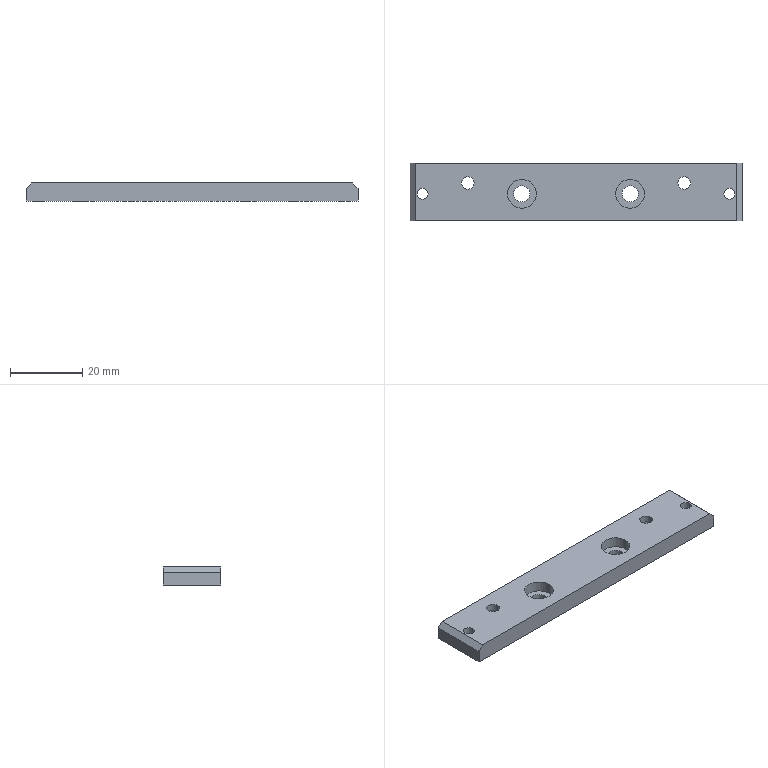NC program | NX | posted with a generic post | part box 92 x 16 x 5 mm
Whole program:
N10 G17 G21 G94 G90
(PLANAR_MILL_COPY , TOOL : D6A45)
N12 T01 M6
N14 G54
N16 G17 G0 G90 X-47.357 Y-8.766 S7500 M3
N18 G43 Z30. H1
N20 Z-1.
N22 G94 G1 Z-2. F1250.
N24 G3 X-47. Y-8. R1.
N26 G1 Y8.
N28 G3 X-47.357 Y8.766 R1.
N30 G1 Z-1.
N32 G0 Z30.
N34 X-46.857 Y-8.766
N36 Z-1.
N38 G1 Z-2.
N40 G3 X-46.5 Y-8. R1.
N42 G1 Y8.
N44 G3 X-46.857 Y8.766 R1.
N46 G1 Z-1.
N48 G0 Z30.
N50 X47.357
N52 Z-1.
N54 G1 Z-2.
N56 G3 X47. Y8. R1.
N58 G1 Y-8.
N60 G3 X47.357 Y-8.766 R1.
N62 G1 Z-1.
N64 G0 Z30.
N66 X46.857 Y8.766
N68 Z-1.
N70 G1 Z-2.
N72 G3 X46.5 Y8. R1.
N74 G1 Y-8.
N76 G3 X46.857 Y-8.766 R1.
N78 G1 Z-1.
N80 G0 Z30.
N82 M5
N84 M2